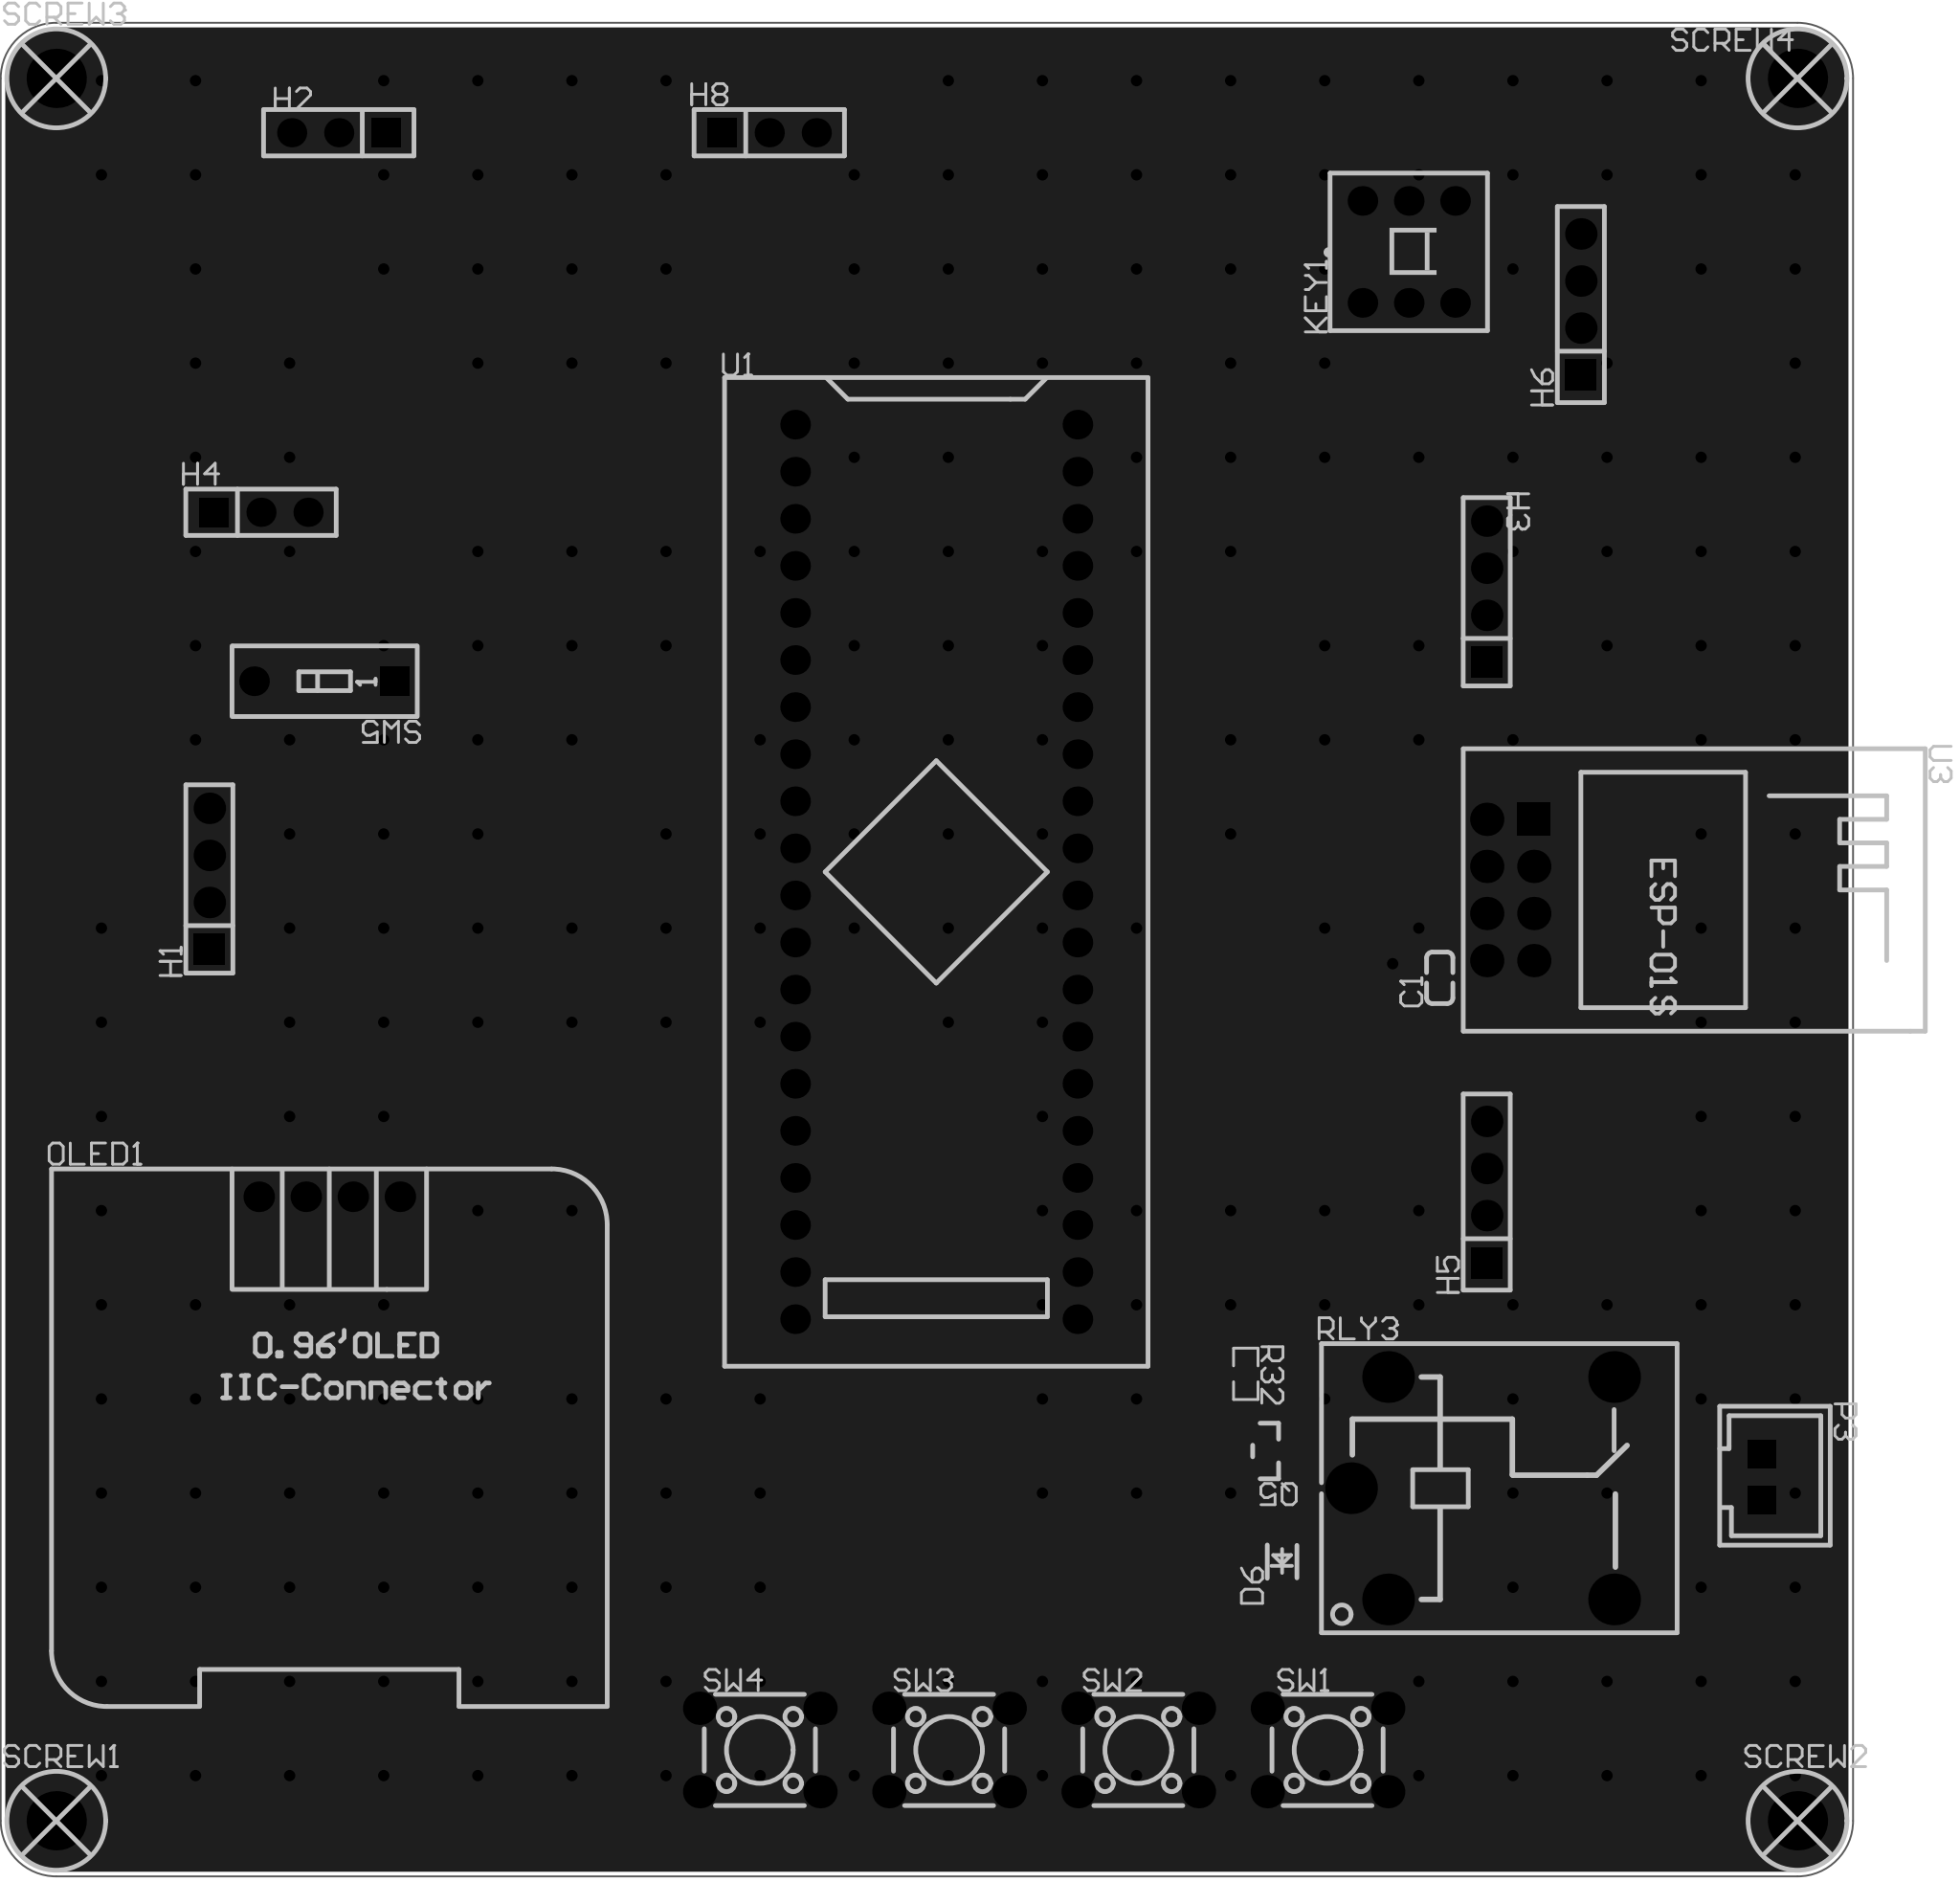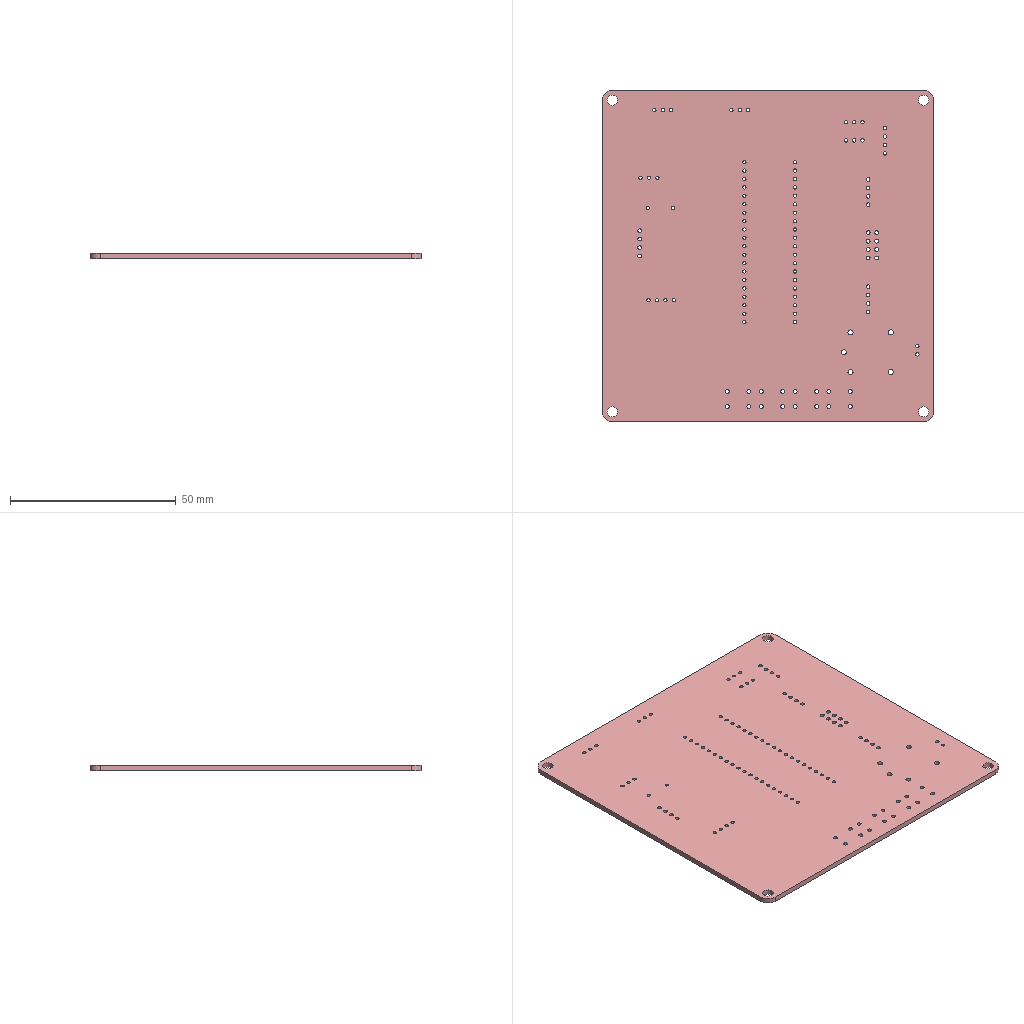Circuit board layout | Altium Designer | box 100 x 100 x 1.6 mm
Layer stack:
# Altium Designer layer stack of  (unit mm; dielectric type: 0 none, 1 core, 2 prepreg, 3 surface material)
index,name,kind,layer,copper_thickness_mm,dielectric_type,dielectric_thickness_mm,dielectric_material,dielectric_constant
0,Top Paste Mask Layer,other,,,,,,
1,Top Silkscreen Layer,other,,,,,,
2,Top Solder Mask Layer,dielectric,,,3,0.01,,3.3
3,Top Layer,copper,Top Layer,0.035,,,,
4,Dielectric1,dielectric,,,3,1.51,FR4,4.5
5,Bottom Layer,copper,Bottom Layer,0.035,,,,
6,Bottom Solder Mask Layer,dielectric,,,3,0.01,,3.3
7,Bottom Silkscreen Layer,other,,,,,,
8,Bottom Paste Mask Layer,other,,,,,,
# drill layer pairs: low layer,high layer
drill_pair,Top Layer,Bottom Layer
Part placement:
Designator,Comment,Layer,Footprint,Center-X(mm),Center-Y(mm),Rotation
H1,,TopLayer,HDR-TH_4P-P2.54-V-M,91.821,132.715,90
H2,,TopLayer,HDR-TH_3P-P2.54-V-F,98.806,172.974,180
H3,,TopLayer,HDR-TH_4P-P2.54-V-M,160.78,148.209,90
H8,,TopLayer,HDR-TH_3P-P2.54-V-F,122.047,172.974,0
KEY1,Non-latching switch 8.5×8.5 silent,TopLayer,SW-TH_6P-L8.5-W8.5-P2.54,156.571,166.545,0
OLED1,,TopLayer,0.96OLED_4P,98.298,115.57,0
U1,STM32F103C8T6-Card,TopLayer,CONN-TH_L53.3-W22.9_STM32F103C8T6-CARD,131.064,133.096,270
SW1,,TopLayer,SW-TH_4P-L6.0-W6.0-P4.50-LS6.5,152.186,85.725,180
SW2,,TopLayer,SW-TH_4P-L6.0-W6.0-P4.50-LS6.5,141.97,85.725,180
SW3,,TopLayer,SW-TH_4P-L6.0-W6.0-P4.50-LS6.5,131.755,85.725,180
SW4,,TopLayer,SW-TH_4P-L6.0-W6.0-P4.50-LS6.5,121.539,85.725,180
C1,1uF,TopLayer,C0603,158.242,127.381,90
D6,LL4148,TopLayer,LL-34_L3.5-W1.5-RD,149.733,95.885,90
H5,,TopLayer,HDR-TH_4P-P2.54-V-F,160.78,115.824,90
P3,XH2.54 through-hole socket-2P,TopLayer,CONN-TH_XH2.54-2P,175.641,100.457,270
Q5,,TopLayer,S8050_SOT-23,148.844,101.854,180
R32,1k,TopLayer,R0603,147.773,106.017,270
RLY3,SRD-05VDC-SL-C,TopLayer,RELAY-TH_SRD-XXVDC-XL-C,160.557,99.846,0
U3,ESP-01S,TopLayer,WIFIM-TH_ESP-01S,162.052,132.121,270
SCREW1,,TopLayer,M3螺丝,83.556,81.905,0
SCREW2,,TopLayer,M3螺丝,177.556,81.905,0
SCREW3,,TopLayer,M3螺丝,83.556,175.905,0
SCREW4,,TopLayer,M3螺丝,177.556,175.905,0
H4,,TopLayer,HDR-TH_3P-P2.54-V-F,94.609,152.498,0
SW5,NDS-01V,TopLayer,SW-TH_2P-L3.9-W9.9-P2.54-LS7.6,98.044,143.383,180
H6,,TopLayer,HDR-TH_4P-P2.54-V-F,165.862,163.703,90
Pad and via stacks:
# Altium Designer via and pad stacks of  (unit mm). Each distinct definition once, with the count of objects using it.
# via: kind,start_layer,end_layer,hole_mm,diameter_mm,mode(0 simple;1 top-mid-bottom;2 full stack),diameter_per_layer,count,example_net
# pad: kind,layer,hole_mm,hole_type(0 round;1 square;2 slot),plating,top_size,top_shape(1 round;2 rect;3 octagon;9 rounded rect),mid_size,bottom_size,mode,footprint,size_per_layer,count,example
pad,Multi-Layer,1.1,0,plated,1.7x1.7,2,1.7x1.7,1.7x1.7,0,HDR-TH_4P-P2.54-V-M,,2,H1.1
pad,Multi-Layer,1.1,0,plated,1.7x1.7,1,1.7x1.7,1.7x1.7,0,HDR-TH_4P-P2.54-V-M,,6,H1.2
pad,Multi-Layer,1.02,0,plated,1.575x1.575,1,1.575x1.575,1.575x1.575,0,HDR-TH_3P-P2.54-V-F,,6,H2.3
pad,Multi-Layer,1.02,0,plated,1.575x1.575,2,1.575x1.575,1.575x1.575,0,HDR-TH_3P-P2.54-V-F,,3,H2.1
pad,Multi-Layer,1,0,plated,1.6x1.6,1,1.6x1.6,1.6x1.6,0,SW-TH_6P-L8.5-W8.5-P2.54,,6,KEY1.4
pad,Multi-Layer,1,0,plated,1.65x1.65,1,1.65x1.65,1.65x1.65,0,0.96OLED_4P,,4,OLED1.4
pad,Multi-Layer,1,0,plated,1.6x1.6,1,1.6x1.6,1.6x1.6,0,CONN-TH_L53.3-W22.9_STM32F103C8T6-CARD,,40,U1.1
pad,Multi-Layer,1.2,0,plated,1.8x1.8,1,1.8x1.8,1.8x1.8,0,SW-TH_4P-L6.0-W6.0-P4.50-LS6.5,,16,SW1.1
pad,Multi-Layer,1.1,0,plated,1.7x1.7,2,1.7x1.7,1.7x1.7,0,HDR-TH_4P-P2.54-V-F,,2,H5.1
pad,Multi-Layer,1.1,0,plated,1.7x1.7,1,1.7x1.7,1.7x1.7,0,HDR-TH_4P-P2.54-V-F,,6,H5.2
pad,Multi-Layer,1,2,plated,1.524x1.524,2,1.524x1.524,1.524x1.524,0,CONN-TH_XH2.54-2P,,2,P3.1
pad,Multi-Layer,1.524,0,plated,2.794x2.794,1,2.794x2.794,2.794x2.794,0,RELAY-TH_SRD-XXVDC-XL-C,,5,RLY3.2
pad,Multi-Layer,1.2,0,plated,1.8x1.8,2,1.8x1.8,1.8x1.8,0,WIFIM-TH_ESP-01S,,1,U3.1
pad,Multi-Layer,1.2,0,plated,1.8x1.8,1,1.8x1.8,1.8x1.8,0,WIFIM-TH_ESP-01S,,7,U3.2
pad,Multi-Layer,3.2,0,plated,3.2x3.2,1,3.2x3.2,3.2x3.2,0,M3\u00C2\u00DD\u00CB\u00BF,,4,SCREW1.1
pad,Multi-Layer,1,0,plated,1.6x1.6,2,1.6x1.6,1.6x1.6,0,SW-TH_2P-L3.9-W9.9-P2.54-LS7.6,,1,SW5.1
pad,Multi-Layer,1,0,plated,1.6x1.6,1,1.6x1.6,1.6x1.6,0,SW-TH_2P-L3.9-W9.9-P2.54-LS7.6,,1,SW5.2
pad,Top Layer,0,0,plated,0.8x0.9,2,0.8x0.9,0.8x0.9,0,C0603,,2,C1.2
pad,Top Layer,0,0,plated,1.1x1.7,2,1.1x1.7,1.1x1.7,0,LL-34_L3.5-W1.5-RD,,2,D6.2
pad,Top Layer,0,0,plated,1x0.8,2,1x0.8,1x0.8,0,S8050_SOT-23,,3,Q5.2
pad,Top Layer,0,0,plated,0.8065x0.864,2,0.8065x0.864,0.8065x0.864,0,R0603,,2,R32.2
via,Top Layer,Bottom Layer,0.3048,0.61,0,,255,VCC
Copper pours:
name,layer,net,type(0 solid;1 hatched;2 none)
Bottom Layer-GND,Bottom Layer,GND,0
Top Layer-GND,Top Layer,GND,0
Design rules, without the lines most boards share:
# Altium Designer design rules of  (exported by Altium Designer, unit mm)
# columns: name | kind | enabled | priority | scope1 | scope2 | descriptor | typed fields (field=value)
copperThickness1oz_2 | 2 | enabled | 2 | All | All | Width Constraint (Min=5mil) (Max=100mil) (Preferred=30mil) (All) |
viaSize | 11 | enabled | 1 | All | All | Routing Via (MinHoleWidth=11.811mil) (MaxHoleWidth=248.032mil) (PreferredHoleWidth=12.008mil) (MinWidth=19.685mil) (MaxWidth=393.701mil) (PreferedWidth=24.016mil) (All) | via_min_hole=0.3 via_max_hole=6.3 via_preferred_diameter=0.61 via_preferred_hole=0.305
solderMaskExpansion | 13 | enabled | 2 | All | All | Solder Mask Expansion (Expansion =2.008mil) (All) | expansion=0.051